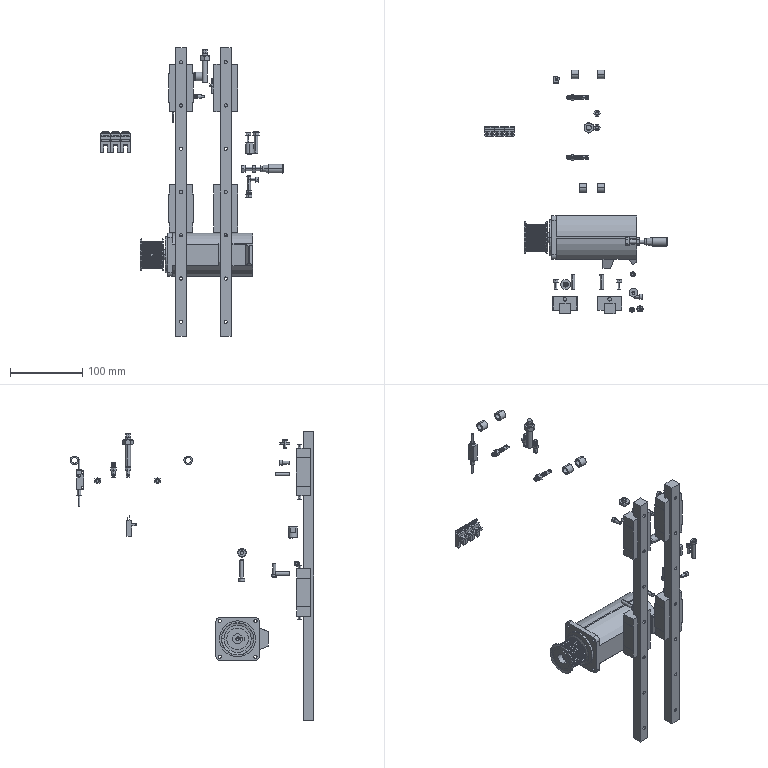Part | NX | 45 solids | 2676 faces | box 253.4 x 337.6 x 400 mm | volume 730031 mm3 | plane 1757 | cylinder 725 | cone 140 | spline 44 | sphere 6 | torus 4 | commonest cylinder face diameters 5 x203 0.5 x52 6.55 x52 1.1 x48 37.24 x48 4.5 x36